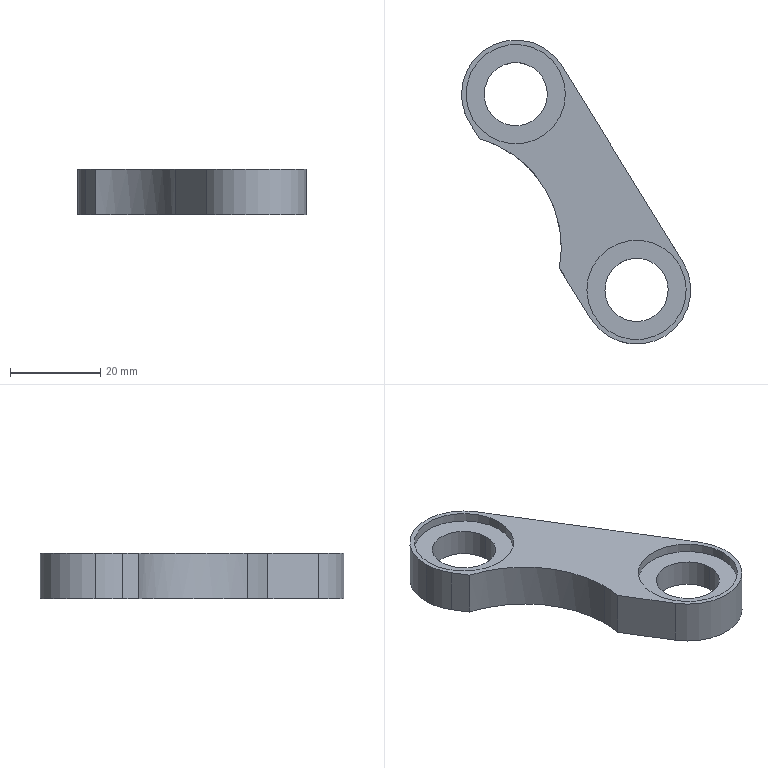Part | SolidWorks | features BaseBody 1 | 1 solid | 26 faces | box 50.743 x 67.323 x 10.007 mm | volume 10354 mm3 | cylinder 17 | plane 9 | commonest cylinder face diameters 22 x8 14 x4 24 x3 50 x2
STEP:
#1=CARTESIAN_POINT('',(366.291,191.387,2.478));
#2=VERTEX_POINT('',#1);
#3=CARTESIAN_POINT('',(388.288,191.747,2.481));
#4=VERTEX_POINT('',#3);
#5=CARTESIAN_POINT('',(377.289,191.567,2.48));
#6=DIRECTION('',(-0.0001435,-0.000000521,1.));
#7=DIRECTION('',(1.,0.,0.0001435));
#8=AXIS2_PLACEMENT_3D('',#5,#6,#7);
#9=CIRCLE('',#8,11.);
#10=EDGE_CURVE('',#2,#4,#9,.T.);
#11=ORIENTED_EDGE('',*,*,#10,.T.);
#12=CARTESIAN_POINT('',(388.288,191.747,0.4812));
#13=VERTEX_POINT('',#12);
#14=CARTESIAN_POINT('',(388.287,191.747,7.281));
#15=DIRECTION('',(0.0001435,0.000000521,-1.));
#16=VECTOR('',#15,1000.);
#17=LINE('',#14,#16);
#18=EDGE_CURVE('',#4,#13,#17,.T.);
#19=ORIENTED_EDGE('',*,*,#18,.T.);
#20=CARTESIAN_POINT('',(366.291,191.387,0.4781));
#21=VERTEX_POINT('',#20);
#22=CARTESIAN_POINT('',(377.29,191.567,0.4797));
#23=DIRECTION('',(-0.0001435,-0.000000521,1.));
#24=DIRECTION('',(-1.,0.,-0.0001435));
#25=AXIS2_PLACEMENT_3D('',#22,#23,#24);
#26=CIRCLE('',#25,11.);
#27=EDGE_CURVE('',#21,#13,#26,.T.);
#28=ORIENTED_EDGE('',*,*,#27,.F.);
#29=CARTESIAN_POINT('',(366.29,191.387,7.278));
#30=DIRECTION('',(0.0001435,0.000000521,-1.));
#31=VECTOR('',#30,1000.);
#32=LINE('',#29,#31);
#33=EDGE_CURVE('',#2,#21,#32,.T.);
#34=ORIENTED_EDGE('',*,*,#33,.F.);
#35=EDGE_LOOP('',(#11,#19,#28,#34));
#36=FACE_OUTER_BOUND('',#35,.T.);
#37=CARTESIAN_POINT('',(377.289,191.567,7.28));
#38=DIRECTION('',(0.0001435,0.000000521,-1.));
#39=DIRECTION('',(-0.9999,-0.01638,-0.0001435));
#40=AXIS2_PLACEMENT_3D('',#37,#38,#39);
#41=CYLINDRICAL_SURFACE('',#40,11.);
#42=ADVANCED_FACE('',(#36),#41,.F.);
#43=CARTESIAN_POINT('',(384.29,191.681,-5.519));
#44=VERTEX_POINT('',#43);
#45=CARTESIAN_POINT('',(370.291,191.452,-5.521));
#46=VERTEX_POINT('',#45);
#47=CARTESIAN_POINT('',(377.29,191.567,-5.52));
#48=DIRECTION('',(-0.0001435,-0.000000521,1.));
#49=DIRECTION('',(-1.,0.,-0.0001435));
#50=AXIS2_PLACEMENT_3D('',#47,#48,#49);
#51=CIRCLE('',#50,7.);
#52=EDGE_CURVE('',#44,#46,#51,.T.);
#53=ORIENTED_EDGE('',*,*,#52,.F.);
#54=CARTESIAN_POINT('',(384.289,191.681,0.4807));
#55=VERTEX_POINT('',#54);
#56=CARTESIAN_POINT('',(384.29,191.681,-9.519));
#57=DIRECTION('',(-0.0001435,-0.000000521,1.));
#58=VECTOR('',#57,1000.);
#59=LINE('',#56,#58);
#60=EDGE_CURVE('',#44,#55,#59,.T.);
#61=ORIENTED_EDGE('',*,*,#60,.T.);
#62=CARTESIAN_POINT('',(370.291,191.452,0.4786));
#63=VERTEX_POINT('',#62);
#64=CARTESIAN_POINT('',(377.29,191.567,0.4797));
#65=DIRECTION('',(0.0001435,0.000000521,-1.));
#66=DIRECTION('',(0.9999,0.01638,0.0001435));
#67=AXIS2_PLACEMENT_3D('',#64,#65,#66);
#68=CIRCLE('',#67,7.);
#69=EDGE_CURVE('',#63,#55,#68,.T.);
#70=ORIENTED_EDGE('',*,*,#69,.F.);
#71=CARTESIAN_POINT('',(370.292,191.452,-9.521));
#72=DIRECTION('',(-0.0001435,-0.000000521,1.));
#73=VECTOR('',#72,1000.);
#74=LINE('',#71,#73);
#75=EDGE_CURVE('',#46,#63,#74,.T.);
#76=ORIENTED_EDGE('',*,*,#75,.F.);
#77=EDGE_LOOP('',(#53,#61,#70,#76));
#78=FACE_OUTER_BOUND('',#77,.T.);
#79=CARTESIAN_POINT('',(377.291,191.567,-9.52));
#80=DIRECTION('',(-0.0001435,-0.000000521,1.));
#81=DIRECTION('',(-0.9999,-0.01638,-0.0001435));
#82=AXIS2_PLACEMENT_3D('',#79,#80,#81);
#83=CYLINDRICAL_SURFACE('',#82,7.);
#84=ADVANCED_FACE('',(#78),#83,.F.);
#85=CARTESIAN_POINT('',(388.289,191.747,-7.519));
#86=VERTEX_POINT('',#85);
#87=CARTESIAN_POINT('',(366.292,191.387,-7.522));
#88=VERTEX_POINT('',#87);
#89=CARTESIAN_POINT('',(377.291,191.567,-7.52));
#90=DIRECTION('',(-0.0001435,-0.000000521,1.));
#91=DIRECTION('',(-1.,0.,-0.0001435));
#92=AXIS2_PLACEMENT_3D('',#89,#90,#91);
#93=CIRCLE('',#92,11.);
#94=EDGE_CURVE('',#86,#88,#93,.T.);
#95=ORIENTED_EDGE('',*,*,#94,.F.);
#96=CARTESIAN_POINT('',(388.289,191.747,-5.519));
#97=VERTEX_POINT('',#96);
#98=CARTESIAN_POINT('',(388.29,191.747,-11.919));
#99=DIRECTION('',(-0.0001435,-0.000000521,1.));
#100=VECTOR('',#99,1000.);
#101=LINE('',#98,#100);
#102=EDGE_CURVE('',#86,#97,#101,.T.);
#103=ORIENTED_EDGE('',*,*,#102,.T.);
#104=CARTESIAN_POINT('',(366.292,191.387,-5.522));
#105=VERTEX_POINT('',#104);
#106=CARTESIAN_POINT('',(377.29,191.567,-5.52));
#107=DIRECTION('',(0.0001435,0.000000521,-1.));
#108=DIRECTION('',(0.9999,0.01638,0.0001435));
#109=AXIS2_PLACEMENT_3D('',#106,#107,#108);
#110=CIRCLE('',#109,11.);
#111=EDGE_CURVE('',#105,#97,#110,.T.);
#112=ORIENTED_EDGE('',*,*,#111,.F.);
#113=CARTESIAN_POINT('',(366.293,191.387,-11.922));
#114=DIRECTION('',(-0.0001435,-0.000000521,1.));
#115=VECTOR('',#114,1000.);
#116=LINE('',#113,#115);
#117=EDGE_CURVE('',#88,#105,#116,.T.);
#118=ORIENTED_EDGE('',*,*,#117,.F.);
#119=EDGE_LOOP('',(#95,#103,#112,#118));
#120=FACE_OUTER_BOUND('',#119,.T.);
#121=CARTESIAN_POINT('',(377.291,191.567,-11.92));
#122=DIRECTION('',(-0.0001435,-0.000000521,1.));
#123=DIRECTION('',(-0.9999,-0.01638,-0.0001435));
#124=AXIS2_PLACEMENT_3D('',#121,#122,#123);
#125=CYLINDRICAL_SURFACE('',#124,11.);
#126=ADVANCED_FACE('',(#120),#125,.F.);
#127=CARTESIAN_POINT('',(360.61,201.025,-7.523));
#128=VERTEX_POINT('',#127);
#129=CARTESIAN_POINT('',(342.52,225.051,-7.525));
#130=VERTEX_POINT('',#129);
#131=CARTESIAN_POINT('',(360.61,201.025,-7.523));
#132=CARTESIAN_POINT('',(360.61,212.602,-7.523));
#133=CARTESIAN_POINT('',(353.647,221.851,-7.524));
#134=CARTESIAN_POINT('',(342.52,225.051,-7.525));
#135=(BOUNDED_CURVE()B_SPLINE_CURVE(3,(#131,#132,#133,#134),.UNSPECIFIED.,.F.,.F.)B_SPLINE_CURVE_WITH_KNOTS((4,4),(6.28,7.57),.UNSPECIFIED.)CURVE()GEOMETRIC_REPRESENTATION_ITEM()RATIONAL_B_SPLINE_CURVE((1.,0.8659,0.8659,1.))REPRESENTATION_ITEM(''));
#136=EDGE_CURVE('',#128,#130,#135,.T.);
#137=ORIENTED_EDGE('',*,*,#136,.F.);
#138=CARTESIAN_POINT('',(360.61,201.025,2.477));
#139=VERTEX_POINT('',#138);
#140=CARTESIAN_POINT('',(360.61,201.025,-10.128));
#141=DIRECTION('',(0.,0.,1.));
#142=VECTOR('',#141,1000.);
#143=LINE('',#140,#142);
#144=EDGE_CURVE('',#128,#139,#143,.T.);
#145=ORIENTED_EDGE('',*,*,#144,.T.);
#146=CARTESIAN_POINT('',(342.519,225.052,2.475));
#147=VERTEX_POINT('',#146);
#148=CARTESIAN_POINT('',(342.519,225.052,2.475));
#149=CARTESIAN_POINT('',(353.646,221.852,2.476));
#150=CARTESIAN_POINT('',(360.61,212.603,2.477));
#151=CARTESIAN_POINT('',(360.61,201.025,2.477));
#152=(BOUNDED_CURVE()B_SPLINE_CURVE(3,(#148,#149,#150,#151),.UNSPECIFIED.,.F.,.F.)B_SPLINE_CURVE_WITH_KNOTS((4,4),(4.996,6.287),.UNSPECIFIED.)CURVE()GEOMETRIC_REPRESENTATION_ITEM()RATIONAL_B_SPLINE_CURVE((1.,0.8659,0.8659,1.))REPRESENTATION_ITEM(''));
#153=EDGE_CURVE('',#147,#139,#152,.T.);
#154=ORIENTED_EDGE('',*,*,#153,.F.);
#155=CARTESIAN_POINT('',(342.519,225.052,2.475));
#156=CARTESIAN_POINT('',(342.52,225.051,-0.8585));
#157=CARTESIAN_POINT('',(342.52,225.051,-4.192));
#158=CARTESIAN_POINT('',(342.52,225.051,-7.525));
#159=B_SPLINE_CURVE_WITH_KNOTS('',3,(#155,#156,#157,#158),.UNSPECIFIED.,.F.,.F.,(4,4),(0.000000606,0.01),.UNSPECIFIED.);
#160=EDGE_CURVE('',#147,#130,#159,.T.);
#161=ORIENTED_EDGE('',*,*,#160,.T.);
#162=EDGE_LOOP('',(#137,#145,#154,#161));
#163=FACE_OUTER_BOUND('',#162,.T.);
#164=CARTESIAN_POINT('',(335.61,201.025,-10.128));
#165=DIRECTION('',(0.,0.,1.));
#166=DIRECTION('',(1.,0.,0.));
#167=AXIS2_PLACEMENT_3D('',#164,#165,#166);
#168=CYLINDRICAL_SURFACE('',#167,25.);
#169=ADVANCED_FACE('',(#163),#168,.F.);
#170=CARTESIAN_POINT('',(338.551,234.694,-7.526));
#171=VERTEX_POINT('',#170);
#172=CARTESIAN_POINT('',(360.761,241.193,-7.523));
#173=VERTEX_POINT('',#172);
#174=CARTESIAN_POINT('',(350.55,234.89,-7.524));
#175=DIRECTION('',(0.0001435,0.000000521,-1.));
#176=DIRECTION('',(-0.851,-0.5252,-0.0001224));
#177=AXIS2_PLACEMENT_3D('',#174,#175,#176);
#178=CIRCLE('',#177,12.);
#179=EDGE_CURVE('',#171,#173,#178,.T.);
#180=ORIENTED_EDGE('',*,*,#179,.F.);
#181=CARTESIAN_POINT('',(338.55,234.693,2.474));
#182=VERTEX_POINT('',#181);
#183=CARTESIAN_POINT('',(338.551,234.694,-9.526));
#184=DIRECTION('',(-0.0001435,-0.000000521,1.));
#185=VECTOR('',#184,1000.);
#186=LINE('',#183,#185);
#187=EDGE_CURVE('',#171,#182,#186,.T.);
#188=ORIENTED_EDGE('',*,*,#187,.T.);
#189=CARTESIAN_POINT('',(360.76,241.193,2.477));
#190=VERTEX_POINT('',#189);
#191=CARTESIAN_POINT('',(350.548,234.89,2.476));
#192=DIRECTION('',(-0.0001435,-0.000000521,1.));
#193=DIRECTION('',(0.851,0.5252,0.0001224));
#194=AXIS2_PLACEMENT_3D('',#191,#192,#193);
#195=CIRCLE('',#194,12.);
#196=EDGE_CURVE('',#190,#182,#195,.T.);
#197=ORIENTED_EDGE('',*,*,#196,.F.);
#198=CARTESIAN_POINT('',(360.76,241.193,2.477));
#199=DIRECTION('',(0.0001435,0.000000521,-1.));
#200=VECTOR('',#199,1000.);
#201=LINE('',#198,#200);
#202=EDGE_CURVE('',#190,#173,#201,.T.);
#203=ORIENTED_EDGE('',*,*,#202,.T.);
#204=EDGE_LOOP('',(#180,#188,#197,#203));
#205=FACE_OUTER_BOUND('',#204,.T.);
#206=CARTESIAN_POINT('',(350.55,234.89,-9.524));
#207=DIRECTION('',(-0.0001435,-0.000000521,1.));
#208=DIRECTION('',(-0.9999,-0.01638,-0.0001435));
#209=AXIS2_PLACEMENT_3D('',#206,#207,#208);
#210=CYLINDRICAL_SURFACE('',#209,12.);
#211=ADVANCED_FACE('',(#205),#210,.T.);
#212=CARTESIAN_POINT('',(361.548,235.07,-7.523));
#213=VERTEX_POINT('',#212);
#214=CARTESIAN_POINT('',(339.551,234.71,-7.526));
#215=VERTEX_POINT('',#214);
#216=CARTESIAN_POINT('',(350.55,234.89,-7.524));
#217=DIRECTION('',(-0.0001435,-0.000000521,1.));
#218=DIRECTION('',(-0.9999,-0.01638,-0.0001435));
#219=AXIS2_PLACEMENT_3D('',#216,#217,#218);
#220=CIRCLE('',#219,11.);
#221=EDGE_CURVE('',#213,#215,#220,.T.);
#222=ORIENTED_EDGE('',*,*,#221,.F.);
#223=CARTESIAN_POINT('',(361.548,235.07,-5.523));
#224=VERTEX_POINT('',#223);
#225=CARTESIAN_POINT('',(361.549,235.07,-11.923));
#226=DIRECTION('',(-0.0001435,-0.000000521,1.));
#227=VECTOR('',#226,1000.);
#228=LINE('',#225,#227);
#229=EDGE_CURVE('',#213,#224,#228,.T.);
#230=ORIENTED_EDGE('',*,*,#229,.T.);
#231=CARTESIAN_POINT('',(339.551,234.71,-5.526));
#232=VERTEX_POINT('',#231);
#233=CARTESIAN_POINT('',(350.549,234.89,-5.524));
#234=DIRECTION('',(0.0001435,0.000000521,-1.));
#235=DIRECTION('',(-1.,0.,-0.0001435));
#236=AXIS2_PLACEMENT_3D('',#233,#234,#235);
#237=CIRCLE('',#236,11.);
#238=EDGE_CURVE('',#232,#224,#237,.T.);
#239=ORIENTED_EDGE('',*,*,#238,.F.);
#240=CARTESIAN_POINT('',(339.552,234.71,-11.926));
#241=DIRECTION('',(-0.0001435,-0.000000521,1.));
#242=VECTOR('',#241,1000.);
#243=LINE('',#240,#242);
#244=EDGE_CURVE('',#215,#232,#243,.T.);
#245=ORIENTED_EDGE('',*,*,#244,.F.);
#246=EDGE_LOOP('',(#222,#230,#239,#245));
#247=FACE_OUTER_BOUND('',#246,.T.);
#248=CARTESIAN_POINT('',(350.55,234.89,-11.924));
#249=DIRECTION('',(-0.0001435,-0.000000521,1.));
#250=DIRECTION('',(-0.9999,-0.01638,-0.0001435));
#251=AXIS2_PLACEMENT_3D('',#248,#249,#250);
#252=CYLINDRICAL_SURFACE('',#251,11.);
#253=ADVANCED_FACE('',(#247),#252,.F.);
#254=CARTESIAN_POINT('',(357.548,235.005,-5.523));
#255=VERTEX_POINT('',#254);
#256=CARTESIAN_POINT('',(343.55,234.775,-5.525));
#257=VERTEX_POINT('',#256);
#258=CARTESIAN_POINT('',(350.549,234.89,-5.524));
#259=DIRECTION('',(-0.0001435,-0.000000521,1.));
#260=DIRECTION('',(-0.9999,-0.01638,-0.0001435));
#261=AXIS2_PLACEMENT_3D('',#258,#259,#260);
#262=CIRCLE('',#261,7.);
#263=EDGE_CURVE('',#255,#257,#262,.T.);
#264=ORIENTED_EDGE('',*,*,#263,.F.);
#265=CARTESIAN_POINT('',(357.547,235.005,0.4768));
#266=VERTEX_POINT('',#265);
#267=CARTESIAN_POINT('',(357.549,235.005,-9.523));
#268=DIRECTION('',(-0.0001435,-0.000000521,1.));
#269=VECTOR('',#268,1000.);
#270=LINE('',#267,#269);
#271=EDGE_CURVE('',#255,#266,#270,.T.);
#272=ORIENTED_EDGE('',*,*,#271,.T.);
#273=CARTESIAN_POINT('',(343.549,234.775,0.4748));
#274=VERTEX_POINT('',#273);
#275=CARTESIAN_POINT('',(350.548,234.89,0.4758));
#276=DIRECTION('',(0.0001435,0.000000521,-1.));
#277=DIRECTION('',(-1.,0.,-0.0001435));
#278=AXIS2_PLACEMENT_3D('',#275,#276,#277);
#279=CIRCLE('',#278,7.);
#280=EDGE_CURVE('',#274,#266,#279,.T.);
#281=ORIENTED_EDGE('',*,*,#280,.F.);
#282=CARTESIAN_POINT('',(343.551,234.775,-9.525));
#283=DIRECTION('',(-0.0001435,-0.000000521,1.));
#284=VECTOR('',#283,1000.);
#285=LINE('',#282,#284);
#286=EDGE_CURVE('',#257,#274,#285,.T.);
#287=ORIENTED_EDGE('',*,*,#286,.F.);
#288=EDGE_LOOP('',(#264,#272,#281,#287));
#289=FACE_OUTER_BOUND('',#288,.T.);
#290=CARTESIAN_POINT('',(350.55,234.89,-9.524));
#291=DIRECTION('',(-0.0001435,-0.000000521,1.));
#292=DIRECTION('',(-0.9999,-0.01638,-0.0001435));
#293=AXIS2_PLACEMENT_3D('',#290,#291,#292);
#294=CYLINDRICAL_SURFACE('',#293,7.);
#295=ADVANCED_FACE('',(#289),#294,.F.);
#296=CARTESIAN_POINT('',(339.55,234.71,2.474));
#297=VERTEX_POINT('',#296);
#298=CARTESIAN_POINT('',(361.547,235.07,2.477));
#299=VERTEX_POINT('',#298);
#300=CARTESIAN_POINT('',(350.548,234.89,2.476));
#301=DIRECTION('',(-0.0001435,-0.000000521,1.));
#302=DIRECTION('',(1.,0.,0.0001435));
#303=AXIS2_PLACEMENT_3D('',#300,#301,#302);
#304=CIRCLE('',#303,11.);
#305=EDGE_CURVE('',#297,#299,#304,.T.);
#306=ORIENTED_EDGE('',*,*,#305,.T.);
#307=CARTESIAN_POINT('',(361.547,235.07,0.4774));
#308=VERTEX_POINT('',#307);
#309=CARTESIAN_POINT('',(361.546,235.07,7.277));
#310=DIRECTION('',(0.0001435,0.000000521,-1.));
#311=VECTOR('',#310,1000.);
#312=LINE('',#309,#311);
#313=EDGE_CURVE('',#299,#308,#312,.T.);
#314=ORIENTED_EDGE('',*,*,#313,.T.);
#315=CARTESIAN_POINT('',(339.55,234.71,0.4743));
#316=VERTEX_POINT('',#315);
#317=CARTESIAN_POINT('',(350.548,234.89,0.4758));
#318=DIRECTION('',(-0.0001435,-0.000000521,1.));
#319=DIRECTION('',(-0.9999,-0.01638,-0.0001435));
#320=AXIS2_PLACEMENT_3D('',#317,#318,#319);
#321=CIRCLE('',#320,11.);
#322=EDGE_CURVE('',#316,#308,#321,.T.);
#323=ORIENTED_EDGE('',*,*,#322,.F.);
#324=CARTESIAN_POINT('',(339.549,234.71,7.274));
#325=DIRECTION('',(0.0001435,0.000000521,-1.));
#326=VECTOR('',#325,1000.);
#327=LINE('',#324,#326);
#328=EDGE_CURVE('',#297,#316,#327,.T.);
#329=ORIENTED_EDGE('',*,*,#328,.F.);
#330=EDGE_LOOP('',(#306,#314,#323,#329));
#331=FACE_OUTER_BOUND('',#330,.T.);
#332=CARTESIAN_POINT('',(350.547,234.89,7.276));
#333=DIRECTION('',(0.0001435,0.000000521,-1.));
#334=DIRECTION('',(-0.9999,-0.01638,-0.0001435));
#335=AXIS2_PLACEMENT_3D('',#332,#333,#334);
#336=CYLINDRICAL_SURFACE('',#335,11.);
#337=ADVANCED_FACE('',(#331),#336,.F.);
#338=ORIENTED_EDGE('',*,*,#313,.F.);
#339=CARTESIAN_POINT('',(350.548,234.89,2.476));
#340=DIRECTION('',(-0.0001435,-0.000000521,1.));
#341=DIRECTION('',(1.,0.,0.0001435));
#342=AXIS2_PLACEMENT_3D('',#339,#340,#341);
#343=CIRCLE('',#342,11.);
#344=EDGE_CURVE('',#299,#297,#343,.T.);
#345=ORIENTED_EDGE('',*,*,#344,.T.);
#346=ORIENTED_EDGE('',*,*,#328,.T.);
#347=CARTESIAN_POINT('',(350.548,234.89,0.4758));
#348=DIRECTION('',(-0.0001435,-0.000000521,1.));
#349=DIRECTION('',(-0.9999,-0.01638,-0.0001435));
#350=AXIS2_PLACEMENT_3D('',#347,#348,#349);
#351=CIRCLE('',#350,11.);
#352=EDGE_CURVE('',#308,#316,#351,.T.);
#353=ORIENTED_EDGE('',*,*,#352,.F.);
#354=EDGE_LOOP('',(#338,#345,#346,#353));
#355=FACE_OUTER_BOUND('',#354,.T.);
#356=CARTESIAN_POINT('',(350.547,234.89,7.276));
#357=DIRECTION('',(0.0001435,0.000000521,-1.));
#358=DIRECTION('',(-0.9999,-0.01638,-0.0001435));
#359=AXIS2_PLACEMENT_3D('',#356,#357,#358);
#360=CYLINDRICAL_SURFACE('',#359,11.);
#361=ADVANCED_FACE('',(#355),#360,.F.);
#362=ORIENTED_EDGE('',*,*,#280,.T.);
#363=CARTESIAN_POINT('',(350.548,234.89,0.4758));
#364=DIRECTION('',(0.0001435,0.000000521,-1.));
#365=DIRECTION('',(-1.,0.,-0.0001435));
#366=AXIS2_PLACEMENT_3D('',#363,#364,#365);
#367=CIRCLE('',#366,7.);
#368=EDGE_CURVE('',#266,#274,#367,.T.);
#369=ORIENTED_EDGE('',*,*,#368,.T.);
#370=EDGE_LOOP('',(#362,#369));
#371=FACE_BOUND('',#370,.T.);
#372=ORIENTED_EDGE('',*,*,#322,.T.);
#373=ORIENTED_EDGE('',*,*,#352,.T.);
#374=EDGE_LOOP('',(#372,#373));
#375=FACE_OUTER_BOUND('',#374,.T.);
#376=CARTESIAN_POINT('',(377.29,191.567,0.4797));
#377=DIRECTION('',(0.0001435,0.000000521,-1.));
#378=DIRECTION('',(0.,-1.,-0.000000521));
#379=AXIS2_PLACEMENT_3D('',#376,#377,#378);
#380=PLANE('',#379);
#381=ADVANCED_FACE('',(#371,#375),#380,.F.);
#382=ORIENTED_EDGE('',*,*,#271,.F.);
#383=CARTESIAN_POINT('',(350.549,234.89,-5.524));
#384=DIRECTION('',(-0.0001435,-0.000000521,1.));
#385=DIRECTION('',(-0.9999,-0.01638,-0.0001435));
#386=AXIS2_PLACEMENT_3D('',#383,#384,#385);
#387=CIRCLE('',#386,7.);
#388=EDGE_CURVE('',#257,#255,#387,.T.);
#389=ORIENTED_EDGE('',*,*,#388,.F.);
#390=ORIENTED_EDGE('',*,*,#286,.T.);
#391=ORIENTED_EDGE('',*,*,#368,.F.);
#392=EDGE_LOOP('',(#382,#389,#390,#391));
#393=FACE_OUTER_BOUND('',#392,.T.);
#394=CARTESIAN_POINT('',(350.55,234.89,-9.524));
#395=DIRECTION('',(-0.0001435,-0.000000521,1.));
#396=DIRECTION('',(-0.9999,-0.01638,-0.0001435));
#397=AXIS2_PLACEMENT_3D('',#394,#395,#396);
#398=CYLINDRICAL_SURFACE('',#397,7.);
#399=ADVANCED_FACE('',(#393),#398,.F.);
#400=ORIENTED_EDGE('',*,*,#388,.T.);
#401=ORIENTED_EDGE('',*,*,#263,.T.);
#402=EDGE_LOOP('',(#400,#401));
#403=FACE_BOUND('',#402,.T.);
#404=ORIENTED_EDGE('',*,*,#238,.T.);
#405=CARTESIAN_POINT('',(350.549,234.89,-5.524));
#406=DIRECTION('',(0.0001435,0.000000521,-1.));
#407=DIRECTION('',(-1.,0.,-0.0001435));
#408=AXIS2_PLACEMENT_3D('',#405,#406,#407);
#409=CIRCLE('',#408,11.);
#410=EDGE_CURVE('',#224,#232,#409,.T.);
#411=ORIENTED_EDGE('',*,*,#410,.T.);
#412=EDGE_LOOP('',(#404,#411));
#413=FACE_OUTER_BOUND('',#412,.T.);
#414=CARTESIAN_POINT('',(377.29,191.567,-5.52));
#415=DIRECTION('',(0.0001435,0.000000521,-1.));
#416=DIRECTION('',(0.,-1.,-0.000000521));
#417=AXIS2_PLACEMENT_3D('',#414,#415,#416);
#418=PLANE('',#417);
#419=ADVANCED_FACE('',(#403,#413),#418,.T.);
#420=ORIENTED_EDGE('',*,*,#229,.F.);
#421=CARTESIAN_POINT('',(350.55,234.89,-7.524));
#422=DIRECTION('',(-0.0001435,-0.000000521,1.));
#423=DIRECTION('',(-0.9999,-0.01638,-0.0001435));
#424=AXIS2_PLACEMENT_3D('',#421,#422,#423);
#425=CIRCLE('',#424,11.);
#426=EDGE_CURVE('',#215,#213,#425,.T.);
#427=ORIENTED_EDGE('',*,*,#426,.F.);
#428=ORIENTED_EDGE('',*,*,#244,.T.);
#429=ORIENTED_EDGE('',*,*,#410,.F.);
#430=EDGE_LOOP('',(#420,#427,#428,#429));
#431=FACE_OUTER_BOUND('',#430,.T.);
#432=CARTESIAN_POINT('',(350.55,234.89,-11.924));
#433=DIRECTION('',(-0.0001435,-0.000000521,1.));
#434=DIRECTION('',(-0.9999,-0.01638,-0.0001435));
#435=AXIS2_PLACEMENT_3D('',#432,#433,#434);
#436=CYLINDRICAL_SURFACE('',#435,11.);
#437=ADVANCED_FACE('',(#431),#436,.F.);
#438=CARTESIAN_POINT('',(367.078,185.264,2.478));
#439=VERTEX_POINT('',#438);
#440=CARTESIAN_POINT('',(367.079,185.264,-7.522));
#441=VERTEX_POINT('',#440);
#442=CARTESIAN_POINT('',(367.078,185.264,2.478));
#443=DIRECTION('',(0.0001435,0.000000521,-1.));
#444=VECTOR('',#443,1000.);
#445=LINE('',#442,#444);
#446=EDGE_CURVE('',#439,#441,#445,.T.);
#447=ORIENTED_EDGE('',*,*,#446,.T.);
#448=CARTESIAN_POINT('',(387.502,197.87,-7.519));
#449=VERTEX_POINT('',#448);
#450=CARTESIAN_POINT('',(377.291,191.567,-7.52));
#451=DIRECTION('',(0.0001435,0.000000521,-1.));
#452=DIRECTION('',(0.851,0.5252,0.0001224));
#453=AXIS2_PLACEMENT_3D('',#450,#451,#452);
#454=CIRCLE('',#453,12.);
#455=EDGE_CURVE('',#449,#441,#454,.T.);
#456=ORIENTED_EDGE('',*,*,#455,.F.);
#457=CARTESIAN_POINT('',(387.501,197.87,2.481));
#458=VERTEX_POINT('',#457);
#459=CARTESIAN_POINT('',(387.502,197.87,-7.519));
#460=DIRECTION('',(-0.0001435,-0.000000521,1.));
#461=VECTOR('',#460,1000.);
#462=LINE('',#459,#461);
#463=EDGE_CURVE('',#449,#458,#462,.T.);
#464=ORIENTED_EDGE('',*,*,#463,.T.);
#465=CARTESIAN_POINT('',(377.289,191.567,2.48));
#466=DIRECTION('',(-0.0001435,-0.000000521,1.));
#467=DIRECTION('',(-0.851,-0.5252,-0.0001224));
#468=AXIS2_PLACEMENT_3D('',#465,#466,#467);
#469=CIRCLE('',#468,12.);
#470=EDGE_CURVE('',#439,#458,#469,.T.);
#471=ORIENTED_EDGE('',*,*,#470,.F.);
#472=EDGE_LOOP('',(#447,#456,#464,#471));
#473=FACE_OUTER_BOUND('',#472,.T.);
#474=CARTESIAN_POINT('',(377.291,191.567,-9.52));
#475=DIRECTION('',(-0.0001435,-0.000000521,1.));
#476=DIRECTION('',(-0.9999,-0.01638,-0.0001435));
#477=AXIS2_PLACEMENT_3D('',#474,#475,#476);
#478=CYLINDRICAL_SURFACE('',#477,12.);
#479=ADVANCED_FACE('',(#473),#478,.T.);
#480=ORIENTED_EDGE('',*,*,#463,.F.);
#481=CARTESIAN_POINT('',(360.761,241.193,-7.523));
#482=DIRECTION('',(0.5252,-0.851,0.00007492));
#483=VECTOR('',#482,1000.);
#484=LINE('',#481,#483);
#485=EDGE_CURVE('',#173,#449,#484,.T.);
#486=ORIENTED_EDGE('',*,*,#485,.F.);
#487=ORIENTED_EDGE('',*,*,#202,.F.);
#488=CARTESIAN_POINT('',(387.501,197.87,2.481));
#489=DIRECTION('',(-0.5252,0.851,-0.00007492));
#490=VECTOR('',#489,1000.);
#491=LINE('',#488,#490);
#492=EDGE_CURVE('',#458,#190,#491,.T.);
#493=ORIENTED_EDGE('',*,*,#492,.F.);
#494=EDGE_LOOP('',(#480,#486,#487,#493));
#495=FACE_OUTER_BOUND('',#494,.T.);
#496=CARTESIAN_POINT('',(387.502,197.87,-9.519));
#497=DIRECTION('',(-0.851,-0.5252,-0.0001224));
#498=DIRECTION('',(-0.5252,0.851,0.));
#499=AXIS2_PLACEMENT_3D('',#496,#497,#498);
#500=PLANE('',#499);
#501=ADVANCED_FACE('',(#495),#500,.F.);
#502=ORIENTED_EDGE('',*,*,#187,.F.);
#503=CARTESIAN_POINT('',(340.338,228.587,-7.526));
#504=VERTEX_POINT('',#503);
#505=CARTESIAN_POINT('',(350.55,234.89,-7.524));
#506=DIRECTION('',(0.0001435,0.000000521,-1.));
#507=DIRECTION('',(-0.851,-0.5252,-0.0001224));
#508=AXIS2_PLACEMENT_3D('',#505,#506,#507);
#509=CIRCLE('',#508,12.);
#510=EDGE_CURVE('',#504,#171,#509,.T.);
#511=ORIENTED_EDGE('',*,*,#510,.F.);
#512=CARTESIAN_POINT('',(340.337,228.587,2.474));
#513=VERTEX_POINT('',#512);
#514=CARTESIAN_POINT('',(340.338,228.587,-7.526));
#515=DIRECTION('',(-0.0001435,-0.000000521,1.));
#516=VECTOR('',#515,1000.);
#517=LINE('',#514,#516);
#518=EDGE_CURVE('',#504,#513,#517,.T.);
#519=ORIENTED_EDGE('',*,*,#518,.T.);
#520=CARTESIAN_POINT('',(350.548,234.89,2.476));
#521=DIRECTION('',(-0.0001435,-0.000000521,1.));
#522=DIRECTION('',(0.851,0.5252,0.0001224));
#523=AXIS2_PLACEMENT_3D('',#520,#521,#522);
#524=CIRCLE('',#523,12.);
#525=EDGE_CURVE('',#182,#513,#524,.T.);
#526=ORIENTED_EDGE('',*,*,#525,.F.);
#527=EDGE_LOOP('',(#502,#511,#519,#526));
#528=FACE_OUTER_BOUND('',#527,.T.);
#529=CARTESIAN_POINT('',(350.55,234.89,-9.524));
#530=DIRECTION('',(-0.0001435,-0.000000521,1.));
#531=DIRECTION('',(-0.9999,-0.01638,-0.0001435));
#532=AXIS2_PLACEMENT_3D('',#529,#530,#531);
#533=CYLINDRICAL_SURFACE('',#532,12.);
#534=ADVANCED_FACE('',(#528),#533,.T.);
#535=ORIENTED_EDGE('',*,*,#160,.F.);
#536=CARTESIAN_POINT('',(367.078,185.264,2.478));
#537=DIRECTION('',(0.5252,-0.851,0.00007492));
#538=VECTOR('',#537,1000.);
#539=LINE('',#536,#538);
#540=EDGE_CURVE('',#513,#147,#539,.T.);
#541=ORIENTED_EDGE('',*,*,#540,.F.);
#542=ORIENTED_EDGE('',*,*,#518,.F.);
#543=CARTESIAN_POINT('',(340.338,228.587,-7.526));
#544=DIRECTION('',(-0.5252,0.851,-0.00007492));
#545=VECTOR('',#544,1000.);
#546=LINE('',#543,#545);
#547=EDGE_CURVE('',#130,#504,#546,.T.);
#548=ORIENTED_EDGE('',*,*,#547,.F.);
#549=EDGE_LOOP('',(#535,#541,#542,#548));
#550=FACE_OUTER_BOUND('',#549,.T.);
#551=CARTESIAN_POINT('',(340.338,228.587,-9.526));
#552=DIRECTION('',(0.851,0.5252,0.0001224));
#553=DIRECTION('',(0.,0.000233,-1.));
#554=AXIS2_PLACEMENT_3D('',#551,#552,#553);
#555=PLANE('',#554);
#556=ADVANCED_FACE('',(#550),#555,.F.);
#557=ORIENTED_EDGE('',*,*,#144,.F.);
#558=CARTESIAN_POINT('',(360.185,196.433,-7.523));
#559=VERTEX_POINT('',#558);
#560=CARTESIAN_POINT('',(360.185,196.433,-7.523));
#561=CARTESIAN_POINT('',(360.468,197.949,-7.523));
#562=CARTESIAN_POINT('',(360.61,199.484,-7.523));
#563=CARTESIAN_POINT('',(360.61,201.025,-7.523));
#564=(BOUNDED_CURVE()B_SPLINE_CURVE(3,(#560,#561,#562,#563),.UNSPECIFIED.,.F.,.F.)B_SPLINE_CURVE_WITH_KNOTS((4,4),(6.095,6.28),.UNSPECIFIED.)CURVE()GEOMETRIC_REPRESENTATION_ITEM()RATIONAL_B_SPLINE_CURVE((1.,0.9972,0.9972,1.))REPRESENTATION_ITEM(''));
#565=EDGE_CURVE('',#559,#128,#564,.T.);
#566=ORIENTED_EDGE('',*,*,#565,.F.);
#567=CARTESIAN_POINT('',(360.185,196.432,2.477));
#568=VERTEX_POINT('',#567);
#569=CARTESIAN_POINT('',(360.185,196.433,-7.523));
#570=CARTESIAN_POINT('',(360.185,196.433,-4.19));
#571=CARTESIAN_POINT('',(360.185,196.432,-0.8563));
#572=CARTESIAN_POINT('',(360.185,196.432,2.477));
#573=B_SPLINE_CURVE_WITH_KNOTS('',3,(#569,#570,#571,#572),.UNSPECIFIED.,.F.,.F.,(4,4),(0.000000233,0.01),.UNSPECIFIED.);
#574=EDGE_CURVE('',#559,#568,#573,.T.);
#575=ORIENTED_EDGE('',*,*,#574,.T.);
#576=CARTESIAN_POINT('',(360.61,201.025,2.477));
#577=CARTESIAN_POINT('',(360.61,199.483,2.477));
#578=CARTESIAN_POINT('',(360.468,197.948,2.477));
#579=CARTESIAN_POINT('',(360.185,196.432,2.477));
#580=(BOUNDED_CURVE()B_SPLINE_CURVE(3,(#576,#577,#578,#579),.UNSPECIFIED.,.F.,.F.)B_SPLINE_CURVE_WITH_KNOTS((4,4),(0.003633,0.1884),.UNSPECIFIED.)CURVE()GEOMETRIC_REPRESENTATION_ITEM()RATIONAL_B_SPLINE_CURVE((1.,0.9972,0.9972,1.))REPRESENTATION_ITEM(''));
#581=EDGE_CURVE('',#139,#568,#580,.T.);
#582=ORIENTED_EDGE('',*,*,#581,.F.);
#583=EDGE_LOOP('',(#557,#566,#575,#582));
#584=FACE_OUTER_BOUND('',#583,.T.);
#585=CARTESIAN_POINT('',(335.61,201.025,-10.128));
#586=DIRECTION('',(0.,0.,1.));
#587=DIRECTION('',(1.,0.,0.));
#588=AXIS2_PLACEMENT_3D('',#585,#586,#587);
#589=CYLINDRICAL_SURFACE('',#588,25.);
#590=ADVANCED_FACE('',(#584),#589,.F.);
#591=ORIENTED_EDGE('',*,*,#426,.T.);
#592=ORIENTED_EDGE('',*,*,#221,.T.);
#593=EDGE_LOOP('',(#591,#592));
#594=FACE_BOUND('',#593,.T.);
#595=CARTESIAN_POINT('',(377.291,191.567,-7.52));
#596=DIRECTION('',(-0.0001435,-0.000000521,1.));
#597=DIRECTION('',(-1.,0.,-0.0001435));
#598=AXIS2_PLACEMENT_3D('',#595,#596,#597);
#599=CIRCLE('',#598,11.);
#600=EDGE_CURVE('',#88,#86,#599,.T.);
#601=ORIENTED_EDGE('',*,*,#600,.T.);
#602=ORIENTED_EDGE('',*,*,#94,.T.);
#603=EDGE_LOOP('',(#601,#602));
#604=FACE_BOUND('',#603,.T.);
#605=ORIENTED_EDGE('',*,*,#547,.T.);
#606=ORIENTED_EDGE('',*,*,#510,.T.);
#607=ORIENTED_EDGE('',*,*,#179,.T.);
#608=ORIENTED_EDGE('',*,*,#485,.T.);
#609=ORIENTED_EDGE('',*,*,#455,.T.);
#610=CARTESIAN_POINT('',(340.338,228.587,-7.526));
#611=DIRECTION('',(-0.5252,0.851,-0.00007492));
#612=VECTOR('',#611,1000.);
#613=LINE('',#610,#612);
#614=EDGE_CURVE('',#441,#559,#613,.T.);
#615=ORIENTED_EDGE('',*,*,#614,.T.);
#616=ORIENTED_EDGE('',*,*,#565,.T.);
#617=ORIENTED_EDGE('',*,*,#136,.T.);
#618=EDGE_LOOP('',(#605,#606,#607,#608,#609,#615,#616,#617));
#619=FACE_OUTER_BOUND('',#618,.T.);
#620=CARTESIAN_POINT('',(377.291,191.567,-7.52));
#621=DIRECTION('',(0.0001435,0.000000521,-1.));
#622=DIRECTION('',(0.,-1.,-0.000000521));
#623=AXIS2_PLACEMENT_3D('',#620,#621,#622);
#624=PLANE('',#623);
#625=ADVANCED_FACE('',(#594,#604,#619),#624,.T.);
#626=ORIENTED_EDGE('',*,*,#102,.F.);
#627=ORIENTED_EDGE('',*,*,#600,.F.);
#628=ORIENTED_EDGE('',*,*,#117,.T.);
#629=CARTESIAN_POINT('',(377.29,191.567,-5.52));
#630=DIRECTION('',(0.0001435,0.000000521,-1.));
#631=DIRECTION('',(0.9999,0.01638,0.0001435));
#632=AXIS2_PLACEMENT_3D('',#629,#630,#631);
#633=CIRCLE('',#632,11.);
#634=EDGE_CURVE('',#97,#105,#633,.T.);
#635=ORIENTED_EDGE('',*,*,#634,.F.);
#636=EDGE_LOOP('',(#626,#627,#628,#635));
#637=FACE_OUTER_BOUND('',#636,.T.);
#638=CARTESIAN_POINT('',(377.291,191.567,-11.92));
#639=DIRECTION('',(-0.0001435,-0.000000521,1.));
#640=DIRECTION('',(-0.9999,-0.01638,-0.0001435));
#641=AXIS2_PLACEMENT_3D('',#638,#639,#640);
#642=CYLINDRICAL_SURFACE('',#641,11.);
#643=ADVANCED_FACE('',(#637),#642,.F.);
#644=CARTESIAN_POINT('',(377.29,191.567,-5.52));
#645=DIRECTION('',(-0.0001435,-0.000000521,1.));
#646=DIRECTION('',(-1.,0.,-0.0001435));
#647=AXIS2_PLACEMENT_3D('',#644,#645,#646);
#648=CIRCLE('',#647,7.);
#649=EDGE_CURVE('',#46,#44,#648,.T.);
#650=ORIENTED_EDGE('',*,*,#649,.T.);
#651=ORIENTED_EDGE('',*,*,#52,.T.);
#652=EDGE_LOOP('',(#650,#651));
#653=FACE_BOUND('',#652,.T.);
#654=ORIENTED_EDGE('',*,*,#111,.T.);
#655=ORIENTED_EDGE('',*,*,#634,.T.);
#656=EDGE_LOOP('',(#654,#655));
#657=FACE_OUTER_BOUND('',#656,.T.);
#658=CARTESIAN_POINT('',(377.29,191.567,-5.52));
#659=DIRECTION('',(0.0001435,0.000000521,-1.));
#660=DIRECTION('',(0.,-1.,-0.000000521));
#661=AXIS2_PLACEMENT_3D('',#658,#659,#660);
#662=PLANE('',#661);
#663=ADVANCED_FACE('',(#653,#657),#662,.T.);
#664=ORIENTED_EDGE('',*,*,#60,.F.);
#665=ORIENTED_EDGE('',*,*,#649,.F.);
#666=ORIENTED_EDGE('',*,*,#75,.T.);
#667=CARTESIAN_POINT('',(377.29,191.567,0.4797));
#668=DIRECTION('',(0.0001435,0.000000521,-1.));
#669=DIRECTION('',(0.9999,0.01638,0.0001435));
#670=AXIS2_PLACEMENT_3D('',#667,#668,#669);
#671=CIRCLE('',#670,7.);
#672=EDGE_CURVE('',#55,#63,#671,.T.);
#673=ORIENTED_EDGE('',*,*,#672,.F.);
#674=EDGE_LOOP('',(#664,#665,#666,#673));
#675=FACE_OUTER_BOUND('',#674,.T.);
#676=CARTESIAN_POINT('',(377.291,191.567,-9.52));
#677=DIRECTION('',(-0.0001435,-0.000000521,1.));
#678=DIRECTION('',(-0.9999,-0.01638,-0.0001435));
#679=AXIS2_PLACEMENT_3D('',#676,#677,#678);
#680=CYLINDRICAL_SURFACE('',#679,7.);
#681=ADVANCED_FACE('',(#675),#680,.F.);
#682=ORIENTED_EDGE('',*,*,#69,.T.);
#683=ORIENTED_EDGE('',*,*,#672,.T.);
#684=EDGE_LOOP('',(#682,#683));
#685=FACE_BOUND('',#684,.T.);
#686=ORIENTED_EDGE('',*,*,#27,.T.);
#687=CARTESIAN_POINT('',(377.29,191.567,0.4797));
#688=DIRECTION('',(-0.0001435,-0.000000521,1.));
#689=DIRECTION('',(-1.,0.,-0.0001435));
#690=AXIS2_PLACEMENT_3D('',#687,#688,#689);
#691=CIRCLE('',#690,11.);
#692=EDGE_CURVE('',#13,#21,#691,.T.);
#693=ORIENTED_EDGE('',*,*,#692,.T.);
#694=EDGE_LOOP('',(#686,#693));
#695=FACE_OUTER_BOUND('',#694,.T.);
#696=CARTESIAN_POINT('',(377.29,191.567,0.4797));
#697=DIRECTION('',(0.0001435,0.000000521,-1.));
#698=DIRECTION('',(0.,-1.,-0.000000521));
#699=AXIS2_PLACEMENT_3D('',#696,#697,#698);
#700=PLANE('',#699);
#701=ADVANCED_FACE('',(#685,#695),#700,.F.);
#702=ORIENTED_EDGE('',*,*,#18,.F.);
#703=CARTESIAN_POINT('',(377.289,191.567,2.48));
#704=DIRECTION('',(-0.0001435,-0.000000521,1.));
#705=DIRECTION('',(1.,0.,0.0001435));
#706=AXIS2_PLACEMENT_3D('',#703,#704,#705);
#707=CIRCLE('',#706,11.);
#708=EDGE_CURVE('',#4,#2,#707,.T.);
#709=ORIENTED_EDGE('',*,*,#708,.T.);
#710=ORIENTED_EDGE('',*,*,#33,.T.);
#711=ORIENTED_EDGE('',*,*,#692,.F.);
#712=EDGE_LOOP('',(#702,#709,#710,#711));
#713=FACE_OUTER_BOUND('',#712,.T.);
#714=CARTESIAN_POINT('',(377.289,191.567,7.28));
#715=DIRECTION('',(0.0001435,0.000000521,-1.));
#716=DIRECTION('',(-0.9999,-0.01638,-0.0001435));
#717=AXIS2_PLACEMENT_3D('',#714,#715,#716);
#718=CYLINDRICAL_SURFACE('',#717,11.);
#719=ADVANCED_FACE('',(#713),#718,.F.);
#720=ORIENTED_EDGE('',*,*,#10,.F.);
#721=ORIENTED_EDGE('',*,*,#708,.F.);
#722=EDGE_LOOP('',(#720,#721));
#723=FACE_BOUND('',#722,.T.);
#724=ORIENTED_EDGE('',*,*,#305,.F.);
#725=ORIENTED_EDGE('',*,*,#344,.F.);
#726=EDGE_LOOP('',(#724,#725));
#727=FACE_BOUND('',#726,.T.);
#728=ORIENTED_EDGE('',*,*,#153,.T.);
#729=ORIENTED_EDGE('',*,*,#581,.T.);
#730=CARTESIAN_POINT('',(367.078,185.264,2.478));
#731=DIRECTION('',(0.5252,-0.851,0.00007492));
#732=VECTOR('',#731,1000.);
#733=LINE('',#730,#732);
#734=EDGE_CURVE('',#568,#439,#733,.T.);
#735=ORIENTED_EDGE('',*,*,#734,.T.);
#736=ORIENTED_EDGE('',*,*,#470,.T.);
#737=ORIENTED_EDGE('',*,*,#492,.T.);
#738=ORIENTED_EDGE('',*,*,#196,.T.);
#739=ORIENTED_EDGE('',*,*,#525,.T.);
#740=ORIENTED_EDGE('',*,*,#540,.T.);
#741=EDGE_LOOP('',(#728,#729,#735,#736,#737,#738,#739,#740));
#742=FACE_OUTER_BOUND('',#741,.T.);
#743=CARTESIAN_POINT('',(377.289,191.567,2.48));
#744=DIRECTION('',(0.0001435,0.000000521,-1.));
#745=DIRECTION('',(0.,-1.,-0.000000521));
#746=AXIS2_PLACEMENT_3D('',#743,#744,#745);
#747=PLANE('',#746);
#748=ADVANCED_FACE('',(#723,#727,#742),#747,.F.);
#749=ORIENTED_EDGE('',*,*,#574,.F.);
#750=ORIENTED_EDGE('',*,*,#614,.F.);
#751=ORIENTED_EDGE('',*,*,#446,.F.);
#752=ORIENTED_EDGE('',*,*,#734,.F.);
#753=EDGE_LOOP('',(#749,#750,#751,#752));
#754=FACE_OUTER_BOUND('',#753,.T.);
#755=CARTESIAN_POINT('',(340.338,228.587,-9.526));
#756=DIRECTION('',(0.851,0.5252,0.0001224));
#757=DIRECTION('',(0.,0.000233,-1.));
#758=AXIS2_PLACEMENT_3D('',#755,#756,#757);
#759=PLANE('',#758);
#760=ADVANCED_FACE('',(#754),#759,.F.);
#761=CLOSED_SHELL('',(#42,#84,#126,#169,#211,#253,#295,#337,#361,#381,#399,#419,#437,#479,#501,#534,#556,#590,#625,#643,#663,#681,#701,#719,#748,#760));
#762=MANIFOLD_SOLID_BREP('',#761);
#763=CARTESIAN_POINT('',(0.,0.,0.));
#764=DIRECTION('',(0.,0.,1.));
#765=DIRECTION('',(1.,0.,0.));
#766=AXIS2_PLACEMENT_3D('',#763,#764,#765);
#767=(LENGTH_UNIT()NAMED_UNIT(*)SI_UNIT(.MILLI.,.METRE.));
#768=UNCERTAINTY_MEASURE_WITH_UNIT(LENGTH_MEASURE(0.00001),#767,'','');
#769=(NAMED_UNIT(*)PLANE_ANGLE_UNIT()SI_UNIT($,.RADIAN.));
#770=(NAMED_UNIT(*)SI_UNIT($,.STERADIAN.)SOLID_ANGLE_UNIT());
#771=(GEOMETRIC_REPRESENTATION_CONTEXT(3)GLOBAL_UNCERTAINTY_ASSIGNED_CONTEXT((#768))GLOBAL_UNIT_ASSIGNED_CONTEXT((#767,#769,#770))REPRESENTATION_CONTEXT('',''));
#772=ADVANCED_BREP_SHAPE_REPRESENTATION('',(#762,#766),#771);